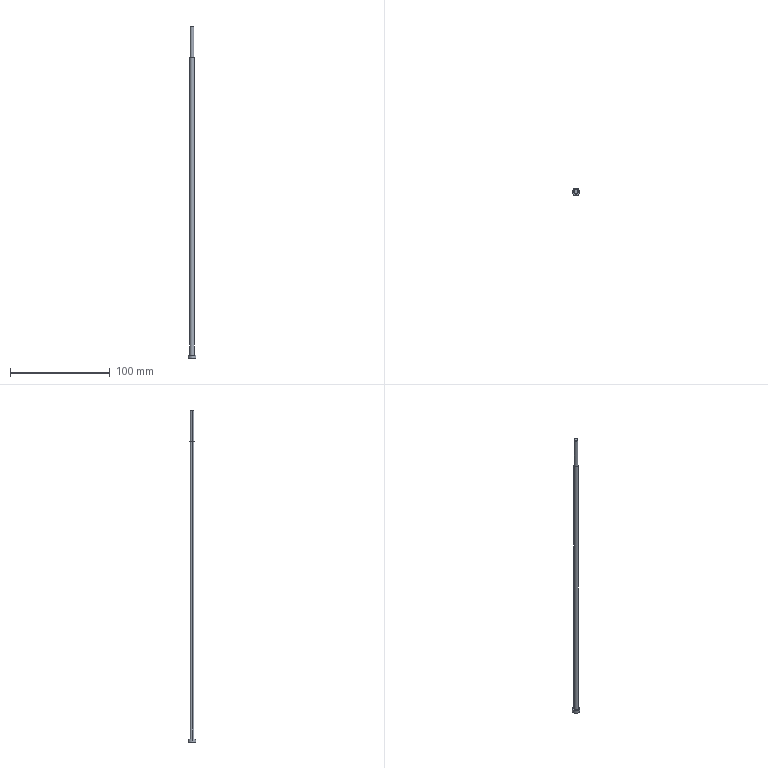Part | Creo | 1 solid | 11 faces | box 8 x 8 x 333.665 mm | volume 5304 mm3 | cylinder 6 | plane 3 | cone 2 | commonest cylinder face diameters 4 x2 4.5 x2 8 x2
STEP:
#1=CARTESIAN_POINT('',(-138.31,238.45,7.486));
#2=VERTEX_POINT('',#1);
#3=CARTESIAN_POINT('',(-142.81,238.45,7.486));
#4=VERTEX_POINT('',#3);
#5=CARTESIAN_POINT('',(-140.56,238.45,7.486));
#6=DIRECTION('',(0.,0.,1.));
#7=DIRECTION('',(1.,0.,0.));
#8=AXIS2_PLACEMENT_3D('',#5,#6,#7);
#9=CIRCLE('',#8,2.25);
#10=EDGE_CURVE('',#2,#4,#9,.T.);
#11=ORIENTED_EDGE('',*,*,#10,.T.);
#12=CARTESIAN_POINT('',(-142.81,238.45,-291.5));
#13=VERTEX_POINT('',#12);
#14=CARTESIAN_POINT('',(-142.81,238.45,-291.5));
#15=DIRECTION('',(0.,0.,1.));
#16=VECTOR('',#15,298.986);
#17=LINE('',#14,#16);
#18=EDGE_CURVE('',#13,#4,#17,.T.);
#19=ORIENTED_EDGE('',*,*,#18,.F.);
#20=CARTESIAN_POINT('',(-138.31,238.45,-291.5));
#21=VERTEX_POINT('',#20);
#22=CARTESIAN_POINT('',(-140.56,238.45,-291.5));
#23=DIRECTION('',(0.,0.,-1.));
#24=DIRECTION('',(-1.,0.,0.));
#25=AXIS2_PLACEMENT_3D('',#22,#23,#24);
#26=CIRCLE('',#25,2.25);
#27=EDGE_CURVE('',#13,#21,#26,.T.);
#28=ORIENTED_EDGE('',*,*,#27,.T.);
#29=CARTESIAN_POINT('',(-138.31,238.45,-291.5));
#30=DIRECTION('',(0.,0.,1.));
#31=VECTOR('',#30,298.986);
#32=LINE('',#29,#31);
#33=EDGE_CURVE('',#21,#2,#32,.T.);
#34=ORIENTED_EDGE('',*,*,#33,.T.);
#35=EDGE_LOOP('',(#11,#19,#28,#34));
#36=FACE_OUTER_BOUND('',#35,.F.);
#37=CARTESIAN_POINT('',(-140.56,238.45,6.697));
#38=DIRECTION('',(0.,0.,1.));
#39=DIRECTION('',(1.,0.,0.));
#40=AXIS2_PLACEMENT_3D('',#37,#38,#39);
#41=CYLINDRICAL_SURFACE('',#40,2.25);
#42=ADVANCED_FACE('',(#36),#41,.T.);
#43=ORIENTED_EDGE('',*,*,#10,.F.);
#44=CARTESIAN_POINT('',(-138.56,238.45,7.736));
#45=VERTEX_POINT('',#44);
#46=CARTESIAN_POINT('',(-138.56,238.45,7.736));
#47=DIRECTION('',(0.7071,0.,-0.7071));
#48=VECTOR('',#47,0.3536);
#49=LINE('',#46,#48);
#50=EDGE_CURVE('',#45,#2,#49,.T.);
#51=ORIENTED_EDGE('',*,*,#50,.F.);
#52=CARTESIAN_POINT('',(-142.56,238.45,7.736));
#53=VERTEX_POINT('',#52);
#54=CARTESIAN_POINT('',(-140.56,238.45,7.736));
#55=DIRECTION('',(0.,0.,-1.));
#56=DIRECTION('',(-1.,0.,0.));
#57=AXIS2_PLACEMENT_3D('',#54,#55,#56);
#58=CIRCLE('',#57,2.);
#59=EDGE_CURVE('',#53,#45,#58,.T.);
#60=ORIENTED_EDGE('',*,*,#59,.F.);
#61=CARTESIAN_POINT('',(-142.56,238.45,7.736));
#62=DIRECTION('',(-0.7071,0.,-0.7071));
#63=VECTOR('',#62,0.3536);
#64=LINE('',#61,#63);
#65=EDGE_CURVE('',#53,#4,#64,.T.);
#66=ORIENTED_EDGE('',*,*,#65,.T.);
#67=EDGE_LOOP('',(#43,#51,#60,#66));
#68=FACE_OUTER_BOUND('',#67,.F.);
#69=CARTESIAN_POINT('',(-140.56,238.45,7.611));
#70=DIRECTION('',(0.,0.,-1.));
#71=DIRECTION('',(-1.,0.,0.));
#72=AXIS2_PLACEMENT_3D('',#69,#70,#71);
#73=CONICAL_SURFACE('',#72,2.125,45.);
#74=ADVANCED_FACE('',(#68),#73,.T.);
#75=CARTESIAN_POINT('',(-140.56,238.45,7.486));
#76=DIRECTION('',(0.,0.,1.));
#77=DIRECTION('',(-1.,0.,0.));
#78=AXIS2_PLACEMENT_3D('',#75,#76,#77);
#79=CIRCLE('',#78,2.25);
#80=EDGE_CURVE('',#4,#2,#79,.T.);
#81=ORIENTED_EDGE('',*,*,#80,.F.);
#82=ORIENTED_EDGE('',*,*,#65,.F.);
#83=CARTESIAN_POINT('',(-140.56,238.45,7.736));
#84=DIRECTION('',(0.,0.,-1.));
#85=DIRECTION('',(1.,0.,0.));
#86=AXIS2_PLACEMENT_3D('',#83,#84,#85);
#87=CIRCLE('',#86,2.);
#88=EDGE_CURVE('',#45,#53,#87,.T.);
#89=ORIENTED_EDGE('',*,*,#88,.F.);
#90=ORIENTED_EDGE('',*,*,#50,.T.);
#91=EDGE_LOOP('',(#81,#82,#89,#90));
#92=FACE_OUTER_BOUND('',#91,.F.);
#93=CARTESIAN_POINT('',(-140.56,238.45,7.611));
#94=DIRECTION('',(0.,0.,-1.));
#95=DIRECTION('',(-1.,0.,0.));
#96=AXIS2_PLACEMENT_3D('',#93,#94,#95);
#97=CONICAL_SURFACE('',#96,2.125,45.);
#98=ADVANCED_FACE('',(#92),#97,.T.);
#99=ORIENTED_EDGE('',*,*,#80,.T.);
#100=ORIENTED_EDGE('',*,*,#33,.F.);
#101=CARTESIAN_POINT('',(-140.56,238.45,-291.5));
#102=DIRECTION('',(0.,0.,-1.));
#103=DIRECTION('',(1.,0.,0.));
#104=AXIS2_PLACEMENT_3D('',#101,#102,#103);
#105=CIRCLE('',#104,2.25);
#106=EDGE_CURVE('',#21,#13,#105,.T.);
#107=ORIENTED_EDGE('',*,*,#106,.T.);
#108=ORIENTED_EDGE('',*,*,#18,.T.);
#109=EDGE_LOOP('',(#99,#100,#107,#108));
#110=FACE_OUTER_BOUND('',#109,.F.);
#111=CARTESIAN_POINT('',(-140.56,238.45,6.697));
#112=DIRECTION('',(0.,0.,1.));
#113=DIRECTION('',(1.,0.,0.));
#114=AXIS2_PLACEMENT_3D('',#111,#112,#113);
#115=CYLINDRICAL_SURFACE('',#114,2.25);
#116=ADVANCED_FACE('',(#110),#115,.T.);
#117=CARTESIAN_POINT('',(-136.56,238.45,-291.5));
#118=VERTEX_POINT('',#117);
#119=CARTESIAN_POINT('',(-144.56,238.45,-291.5));
#120=VERTEX_POINT('',#119);
#121=CARTESIAN_POINT('',(-140.56,238.45,-291.5));
#122=DIRECTION('',(0.,0.,1.));
#123=DIRECTION('',(1.,0.,0.));
#124=AXIS2_PLACEMENT_3D('',#121,#122,#123);
#125=CIRCLE('',#124,4.);
#126=EDGE_CURVE('',#118,#120,#125,.T.);
#127=ORIENTED_EDGE('',*,*,#126,.F.);
#128=CARTESIAN_POINT('',(-140.56,238.45,-291.5));
#129=DIRECTION('',(0.,0.,1.));
#130=DIRECTION('',(-1.,0.,0.));
#131=AXIS2_PLACEMENT_3D('',#128,#129,#130);
#132=CIRCLE('',#131,4.);
#133=EDGE_CURVE('',#120,#118,#132,.T.);
#134=ORIENTED_EDGE('',*,*,#133,.F.);
#135=EDGE_LOOP('',(#127,#134));
#136=FACE_OUTER_BOUND('',#135,.F.);
#137=ORIENTED_EDGE('',*,*,#106,.F.);
#138=ORIENTED_EDGE('',*,*,#27,.F.);
#139=EDGE_LOOP('',(#137,#138));
#140=FACE_BOUND('',#139,.F.);
#141=CARTESIAN_POINT('',(-140.56,238.45,-291.5));
#142=DIRECTION('',(0.,0.,1.));
#143=DIRECTION('',(-1.,0.,0.));
#144=AXIS2_PLACEMENT_3D('',#141,#142,#143);
#145=PLANE('',#144);
#146=ADVANCED_FACE('',(#136,#140),#145,.T.);
#147=ORIENTED_EDGE('',*,*,#126,.T.);
#148=CARTESIAN_POINT('',(-144.56,238.45,-294.5));
#149=VERTEX_POINT('',#148);
#150=CARTESIAN_POINT('',(-144.56,238.45,-294.5));
#151=DIRECTION('',(0.,0.,1.));
#152=VECTOR('',#151,3.);
#153=LINE('',#150,#152);
#154=EDGE_CURVE('',#149,#120,#153,.T.);
#155=ORIENTED_EDGE('',*,*,#154,.F.);
#156=CARTESIAN_POINT('',(-136.56,238.45,-294.5));
#157=VERTEX_POINT('',#156);
#158=CARTESIAN_POINT('',(-140.56,238.45,-294.5));
#159=DIRECTION('',(0.,0.,-1.));
#160=DIRECTION('',(-1.,0.,0.));
#161=AXIS2_PLACEMENT_3D('',#158,#159,#160);
#162=CIRCLE('',#161,4.);
#163=EDGE_CURVE('',#149,#157,#162,.T.);
#164=ORIENTED_EDGE('',*,*,#163,.T.);
#165=CARTESIAN_POINT('',(-136.56,238.45,-294.5));
#166=DIRECTION('',(0.,0.,1.));
#167=VECTOR('',#166,3.);
#168=LINE('',#165,#167);
#169=EDGE_CURVE('',#157,#118,#168,.T.);
#170=ORIENTED_EDGE('',*,*,#169,.T.);
#171=EDGE_LOOP('',(#147,#155,#164,#170));
#172=FACE_OUTER_BOUND('',#171,.F.);
#173=CARTESIAN_POINT('',(-140.56,238.45,-294.5));
#174=DIRECTION('',(0.,0.,1.));
#175=DIRECTION('',(-1.,0.,0.));
#176=AXIS2_PLACEMENT_3D('',#173,#174,#175);
#177=CYLINDRICAL_SURFACE('',#176,4.);
#178=ADVANCED_FACE('',(#172),#177,.T.);
#179=ORIENTED_EDGE('',*,*,#133,.T.);
#180=ORIENTED_EDGE('',*,*,#169,.F.);
#181=CARTESIAN_POINT('',(-140.56,238.45,-294.5));
#182=DIRECTION('',(0.,0.,-1.));
#183=DIRECTION('',(1.,0.,0.));
#184=AXIS2_PLACEMENT_3D('',#181,#182,#183);
#185=CIRCLE('',#184,4.);
#186=EDGE_CURVE('',#157,#149,#185,.T.);
#187=ORIENTED_EDGE('',*,*,#186,.T.);
#188=ORIENTED_EDGE('',*,*,#154,.T.);
#189=EDGE_LOOP('',(#179,#180,#187,#188));
#190=FACE_OUTER_BOUND('',#189,.F.);
#191=CARTESIAN_POINT('',(-140.56,238.45,-294.5));
#192=DIRECTION('',(0.,0.,1.));
#193=DIRECTION('',(-1.,0.,0.));
#194=AXIS2_PLACEMENT_3D('',#191,#192,#193);
#195=CYLINDRICAL_SURFACE('',#194,4.);
#196=ADVANCED_FACE('',(#190),#195,.T.);
#197=ORIENTED_EDGE('',*,*,#163,.F.);
#198=ORIENTED_EDGE('',*,*,#186,.F.);
#199=EDGE_LOOP('',(#197,#198));
#200=FACE_OUTER_BOUND('',#199,.F.);
#201=CARTESIAN_POINT('',(372.125,-398.228,-294.5));
#202=DIRECTION('',(0.,0.,-1.));
#203=DIRECTION('',(1.,0.,0.));
#204=AXIS2_PLACEMENT_3D('',#201,#202,#203);
#205=PLANE('',#204);
#206=ADVANCED_FACE('',(#200),#205,.T.);
#207=CARTESIAN_POINT('',(-142.56,238.45,39.165));
#208=VERTEX_POINT('',#207);
#209=CARTESIAN_POINT('',(-138.56,238.45,39.165));
#210=VERTEX_POINT('',#209);
#211=CARTESIAN_POINT('',(-140.56,238.45,39.165));
#212=DIRECTION('',(0.,0.,1.));
#213=DIRECTION('',(-1.,0.,0.));
#214=AXIS2_PLACEMENT_3D('',#211,#212,#213);
#215=CIRCLE('',#214,2.);
#216=EDGE_CURVE('',#208,#210,#215,.T.);
#217=ORIENTED_EDGE('',*,*,#216,.T.);
#218=CARTESIAN_POINT('',(-138.56,238.45,7.736));
#219=DIRECTION('',(0.,0.,1.));
#220=VECTOR('',#219,31.429);
#221=LINE('',#218,#220);
#222=EDGE_CURVE('',#45,#210,#221,.T.);
#223=ORIENTED_EDGE('',*,*,#222,.F.);
#224=ORIENTED_EDGE('',*,*,#88,.T.);
#225=CARTESIAN_POINT('',(-142.56,238.45,7.736));
#226=DIRECTION('',(0.,0.,1.));
#227=VECTOR('',#226,31.429);
#228=LINE('',#225,#227);
#229=EDGE_CURVE('',#53,#208,#228,.T.);
#230=ORIENTED_EDGE('',*,*,#229,.T.);
#231=EDGE_LOOP('',(#217,#223,#224,#230));
#232=FACE_OUTER_BOUND('',#231,.F.);
#233=CARTESIAN_POINT('',(-140.56,238.45,6.697));
#234=DIRECTION('',(0.,0.,1.));
#235=DIRECTION('',(1.,0.,0.));
#236=AXIS2_PLACEMENT_3D('',#233,#234,#235);
#237=CYLINDRICAL_SURFACE('',#236,2.);
#238=ADVANCED_FACE('',(#232),#237,.T.);
#239=ORIENTED_EDGE('',*,*,#216,.F.);
#240=CARTESIAN_POINT('',(-140.56,238.45,39.165));
#241=DIRECTION('',(0.,0.,1.));
#242=DIRECTION('',(1.,0.,0.));
#243=AXIS2_PLACEMENT_3D('',#240,#241,#242);
#244=CIRCLE('',#243,2.);
#245=EDGE_CURVE('',#210,#208,#244,.T.);
#246=ORIENTED_EDGE('',*,*,#245,.F.);
#247=EDGE_LOOP('',(#239,#246));
#248=FACE_OUTER_BOUND('',#247,.F.);
#249=CARTESIAN_POINT('',(0.,0.,39.165));
#250=DIRECTION('',(0.,0.,-1.));
#251=DIRECTION('',(0.,1.,0.));
#252=AXIS2_PLACEMENT_3D('',#249,#250,#251);
#253=PLANE('',#252);
#254=ADVANCED_FACE('',(#248),#253,.F.);
#255=ORIENTED_EDGE('',*,*,#245,.T.);
#256=ORIENTED_EDGE('',*,*,#229,.F.);
#257=ORIENTED_EDGE('',*,*,#59,.T.);
#258=ORIENTED_EDGE('',*,*,#222,.T.);
#259=EDGE_LOOP('',(#255,#256,#257,#258));
#260=FACE_OUTER_BOUND('',#259,.F.);
#261=CARTESIAN_POINT('',(-140.56,238.45,6.697));
#262=DIRECTION('',(0.,0.,1.));
#263=DIRECTION('',(1.,0.,0.));
#264=AXIS2_PLACEMENT_3D('',#261,#262,#263);
#265=CYLINDRICAL_SURFACE('',#264,2.);
#266=ADVANCED_FACE('',(#260),#265,.T.);
#267=CLOSED_SHELL('',(#42,#74,#98,#116,#146,#178,#196,#206,#238,#254,#266));
#268=MANIFOLD_SOLID_BREP('',#267);
#269=(LENGTH_UNIT()NAMED_UNIT(*)SI_UNIT(.MILLI.,.METRE.));
#270=UNCERTAINTY_MEASURE_WITH_UNIT(LENGTH_MEASURE(0.03338),#269,'','');
#271=(NAMED_UNIT(*)PLANE_ANGLE_UNIT()SI_UNIT($,.RADIAN.));
#272=PLANE_ANGLE_MEASURE_WITH_UNIT(PLANE_ANGLE_MEASURE(0.01745),#271);
#273=(CONVERSION_BASED_UNIT('DEGREE',#272)NAMED_UNIT(*)PLANE_ANGLE_UNIT());
#274=(NAMED_UNIT(*)SI_UNIT($,.STERADIAN.)SOLID_ANGLE_UNIT());
#275=(GEOMETRIC_REPRESENTATION_CONTEXT(3)GLOBAL_UNCERTAINTY_ASSIGNED_CONTEXT((#270))GLOBAL_UNIT_ASSIGNED_CONTEXT((#269,#273,#274))REPRESENTATION_CONTEXT('',''));
#276=ADVANCED_BREP_SHAPE_REPRESENTATION('',(#268),#275);